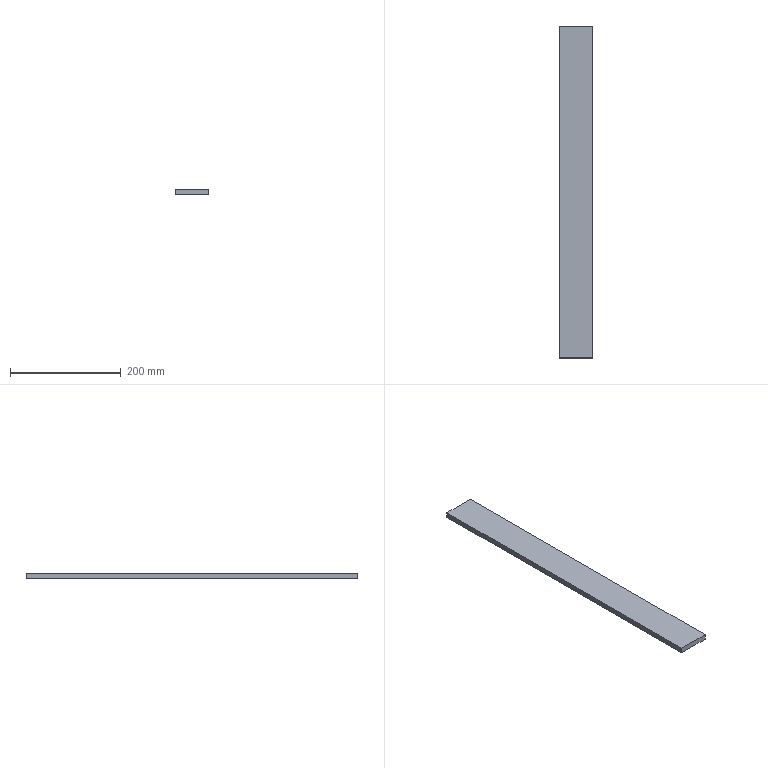Part | SolidWorks | features Extrusion 1 | 1 solid | 6 faces | box 60 x 600 x 10 mm | volume 360000 mm3 | plane 6
STEP:
#1=CARTESIAN_POINT('',(0.,600.,0.));
#2=VERTEX_POINT('',#1);
#3=CARTESIAN_POINT('',(0.,0.,0.));
#4=VERTEX_POINT('',#3);
#5=CARTESIAN_POINT('',(0.,0.,0.));
#6=DIRECTION('',(0.,-1.,0.));
#7=VECTOR('',#6,1000.);
#8=LINE('',#5,#7);
#9=EDGE_CURVE('',#2,#4,#8,.T.);
#10=ORIENTED_EDGE('',*,*,#9,.T.);
#11=CARTESIAN_POINT('',(0.,0.,10.));
#12=VERTEX_POINT('',#11);
#13=CARTESIAN_POINT('',(0.,0.,10.));
#14=DIRECTION('',(0.,0.,-1.));
#15=VECTOR('',#14,1000.);
#16=LINE('',#13,#15);
#17=EDGE_CURVE('',#12,#4,#16,.T.);
#18=ORIENTED_EDGE('',*,*,#17,.F.);
#19=CARTESIAN_POINT('',(0.,600.,10.));
#20=VERTEX_POINT('',#19);
#21=CARTESIAN_POINT('',(0.,0.,10.));
#22=DIRECTION('',(0.,-1.,0.));
#23=VECTOR('',#22,1000.);
#24=LINE('',#21,#23);
#25=EDGE_CURVE('',#20,#12,#24,.T.);
#26=ORIENTED_EDGE('',*,*,#25,.F.);
#27=CARTESIAN_POINT('',(0.,600.,10.));
#28=DIRECTION('',(0.,0.,-1.));
#29=VECTOR('',#28,1000.);
#30=LINE('',#27,#29);
#31=EDGE_CURVE('',#20,#2,#30,.T.);
#32=ORIENTED_EDGE('',*,*,#31,.T.);
#33=EDGE_LOOP('',(#10,#18,#26,#32));
#34=FACE_OUTER_BOUND('',#33,.T.);
#35=CARTESIAN_POINT('',(0.,0.,10.));
#36=DIRECTION('',(1.,0.,0.));
#37=DIRECTION('',(0.,1.,0.));
#38=AXIS2_PLACEMENT_3D('',#35,#36,#37);
#39=PLANE('',#38);
#40=ADVANCED_FACE('',(#34),#39,.F.);
#41=CARTESIAN_POINT('',(60.,0.,0.));
#42=VERTEX_POINT('',#41);
#43=CARTESIAN_POINT('',(0.,0.,0.));
#44=DIRECTION('',(1.,0.,0.));
#45=VECTOR('',#44,1000.);
#46=LINE('',#43,#45);
#47=EDGE_CURVE('',#4,#42,#46,.T.);
#48=ORIENTED_EDGE('',*,*,#47,.T.);
#49=CARTESIAN_POINT('',(60.,0.,10.));
#50=VERTEX_POINT('',#49);
#51=CARTESIAN_POINT('',(60.,0.,10.));
#52=DIRECTION('',(0.,0.,-1.));
#53=VECTOR('',#52,1000.);
#54=LINE('',#51,#53);
#55=EDGE_CURVE('',#50,#42,#54,.T.);
#56=ORIENTED_EDGE('',*,*,#55,.F.);
#57=CARTESIAN_POINT('',(0.,0.,10.));
#58=DIRECTION('',(1.,0.,0.));
#59=VECTOR('',#58,1000.);
#60=LINE('',#57,#59);
#61=EDGE_CURVE('',#12,#50,#60,.T.);
#62=ORIENTED_EDGE('',*,*,#61,.F.);
#63=ORIENTED_EDGE('',*,*,#17,.T.);
#64=EDGE_LOOP('',(#48,#56,#62,#63));
#65=FACE_OUTER_BOUND('',#64,.T.);
#66=CARTESIAN_POINT('',(0.,0.,10.));
#67=DIRECTION('',(0.,1.,0.));
#68=DIRECTION('',(0.,0.,1.));
#69=AXIS2_PLACEMENT_3D('',#66,#67,#68);
#70=PLANE('',#69);
#71=ADVANCED_FACE('',(#65),#70,.F.);
#72=CARTESIAN_POINT('',(60.,600.,0.));
#73=VERTEX_POINT('',#72);
#74=CARTESIAN_POINT('',(60.,0.,0.));
#75=DIRECTION('',(0.,1.,0.));
#76=VECTOR('',#75,1000.);
#77=LINE('',#74,#76);
#78=EDGE_CURVE('',#42,#73,#77,.T.);
#79=ORIENTED_EDGE('',*,*,#78,.T.);
#80=CARTESIAN_POINT('',(60.,600.,10.));
#81=VERTEX_POINT('',#80);
#82=CARTESIAN_POINT('',(60.,600.,10.));
#83=DIRECTION('',(0.,0.,-1.));
#84=VECTOR('',#83,1000.);
#85=LINE('',#82,#84);
#86=EDGE_CURVE('',#81,#73,#85,.T.);
#87=ORIENTED_EDGE('',*,*,#86,.F.);
#88=CARTESIAN_POINT('',(60.,0.,10.));
#89=DIRECTION('',(0.,1.,0.));
#90=VECTOR('',#89,1000.);
#91=LINE('',#88,#90);
#92=EDGE_CURVE('',#50,#81,#91,.T.);
#93=ORIENTED_EDGE('',*,*,#92,.F.);
#94=ORIENTED_EDGE('',*,*,#55,.T.);
#95=EDGE_LOOP('',(#79,#87,#93,#94));
#96=FACE_OUTER_BOUND('',#95,.T.);
#97=CARTESIAN_POINT('',(60.,0.,10.));
#98=DIRECTION('',(-1.,0.,0.));
#99=DIRECTION('',(0.,-1.,0.));
#100=AXIS2_PLACEMENT_3D('',#97,#98,#99);
#101=PLANE('',#100);
#102=ADVANCED_FACE('',(#96),#101,.F.);
#103=CARTESIAN_POINT('',(0.,600.,0.));
#104=DIRECTION('',(-1.,0.,0.));
#105=VECTOR('',#104,1000.);
#106=LINE('',#103,#105);
#107=EDGE_CURVE('',#73,#2,#106,.T.);
#108=ORIENTED_EDGE('',*,*,#107,.T.);
#109=ORIENTED_EDGE('',*,*,#31,.F.);
#110=CARTESIAN_POINT('',(0.,600.,10.));
#111=DIRECTION('',(-1.,0.,0.));
#112=VECTOR('',#111,1000.);
#113=LINE('',#110,#112);
#114=EDGE_CURVE('',#81,#20,#113,.T.);
#115=ORIENTED_EDGE('',*,*,#114,.F.);
#116=ORIENTED_EDGE('',*,*,#86,.T.);
#117=EDGE_LOOP('',(#108,#109,#115,#116));
#118=FACE_OUTER_BOUND('',#117,.T.);
#119=CARTESIAN_POINT('',(0.,600.,10.));
#120=DIRECTION('',(0.,-1.,0.));
#121=DIRECTION('',(0.,0.,-1.));
#122=AXIS2_PLACEMENT_3D('',#119,#120,#121);
#123=PLANE('',#122);
#124=ADVANCED_FACE('',(#118),#123,.F.);
#125=ORIENTED_EDGE('',*,*,#25,.T.);
#126=ORIENTED_EDGE('',*,*,#61,.T.);
#127=ORIENTED_EDGE('',*,*,#92,.T.);
#128=ORIENTED_EDGE('',*,*,#114,.T.);
#129=EDGE_LOOP('',(#125,#126,#127,#128));
#130=FACE_OUTER_BOUND('',#129,.T.);
#131=CARTESIAN_POINT('',(0.,0.,10.));
#132=DIRECTION('',(0.,0.,-1.));
#133=DIRECTION('',(-1.,0.,0.));
#134=AXIS2_PLACEMENT_3D('',#131,#132,#133);
#135=PLANE('',#134);
#136=ADVANCED_FACE('',(#130),#135,.F.);
#137=ORIENTED_EDGE('',*,*,#9,.F.);
#138=ORIENTED_EDGE('',*,*,#107,.F.);
#139=ORIENTED_EDGE('',*,*,#78,.F.);
#140=ORIENTED_EDGE('',*,*,#47,.F.);
#141=EDGE_LOOP('',(#137,#138,#139,#140));
#142=FACE_OUTER_BOUND('',#141,.T.);
#143=CARTESIAN_POINT('',(0.,0.,0.));
#144=DIRECTION('',(0.,0.,-1.));
#145=DIRECTION('',(-1.,0.,0.));
#146=AXIS2_PLACEMENT_3D('',#143,#144,#145);
#147=PLANE('',#146);
#148=ADVANCED_FACE('',(#142),#147,.T.);
#149=CLOSED_SHELL('',(#40,#71,#102,#124,#136,#148));
#150=MANIFOLD_SOLID_BREP('',#149);
#151=CARTESIAN_POINT('',(0.,0.,0.));
#152=DIRECTION('',(0.,0.,1.));
#153=DIRECTION('',(1.,0.,0.));
#154=AXIS2_PLACEMENT_3D('',#151,#152,#153);
#155=(LENGTH_UNIT()NAMED_UNIT(*)SI_UNIT(.MILLI.,.METRE.));
#156=UNCERTAINTY_MEASURE_WITH_UNIT(LENGTH_MEASURE(0.00001),#155,'','');
#157=(NAMED_UNIT(*)PLANE_ANGLE_UNIT()SI_UNIT($,.RADIAN.));
#158=(NAMED_UNIT(*)SI_UNIT($,.STERADIAN.)SOLID_ANGLE_UNIT());
#159=(GEOMETRIC_REPRESENTATION_CONTEXT(3)GLOBAL_UNCERTAINTY_ASSIGNED_CONTEXT((#156))GLOBAL_UNIT_ASSIGNED_CONTEXT((#155,#157,#158))REPRESENTATION_CONTEXT('',''));
#160=ADVANCED_BREP_SHAPE_REPRESENTATION('',(#150,#154),#159);